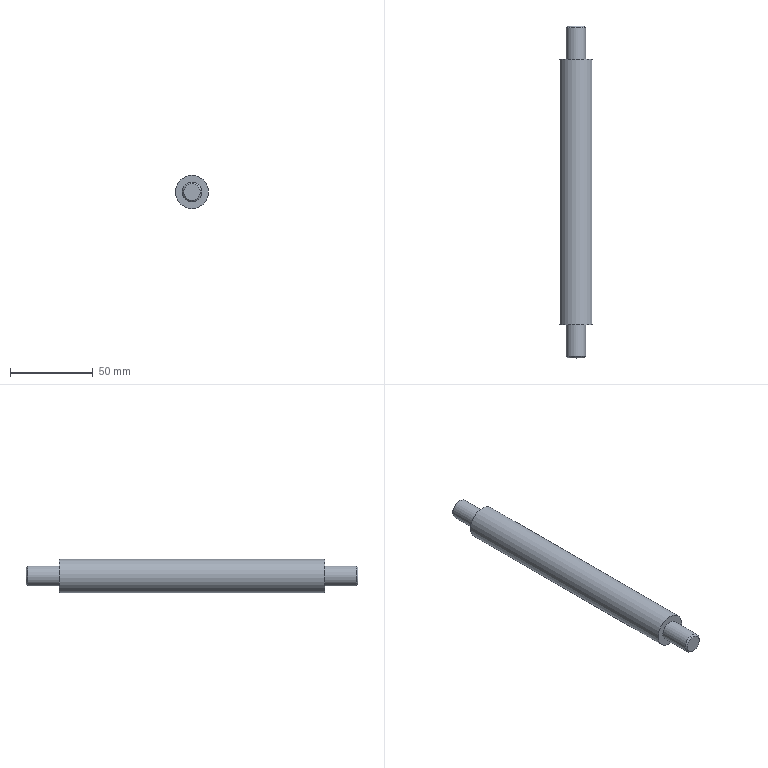Part | STEP file | 冲床-300配套压波_id754_x_t | 1 solid | 9 faces | box 20 x 200 x 20 mm | volume 54754 mm3 | plane 4 | cylinder 3 | cone 2 | commonest cylinder face diameters 12 x2 20 x1
STEP:
#1=CARTESIAN_POINT('',(1915.,80.,68.));
#2=VERTEX_POINT('',#1);
#3=CARTESIAN_POINT('',(1915.,80.,58.));
#4=DIRECTION('',(0.,1.,0.));
#5=DIRECTION('',(0.,0.,1.));
#6=AXIS2_PLACEMENT_3D('',#3,#4,#5);
#7=CIRCLE('',#6,10.);
#8=EDGE_CURVE('',#2,#2,#7,.T.);
#9=ORIENTED_EDGE('',*,*,#8,.F.);
#10=EDGE_LOOP('',(#9));
#11=FACE_BOUND('',#10,.T.);
#12=CARTESIAN_POINT('',(1915.,-80.,48.));
#13=VERTEX_POINT('',#12);
#14=CARTESIAN_POINT('',(1915.,-80.,58.));
#15=DIRECTION('',(0.,-1.,0.));
#16=DIRECTION('',(0.,0.,-1.));
#17=AXIS2_PLACEMENT_3D('',#14,#15,#16);
#18=CIRCLE('',#17,10.);
#19=EDGE_CURVE('',#13,#13,#18,.T.);
#20=ORIENTED_EDGE('',*,*,#19,.F.);
#21=EDGE_LOOP('',(#20));
#22=FACE_BOUND('',#21,.T.);
#23=CARTESIAN_POINT('',(1915.,-45.,58.));
#24=DIRECTION('',(0.,1.,0.));
#25=DIRECTION('',(0.,0.,-1.));
#26=AXIS2_PLACEMENT_3D('',#23,#24,#25);
#27=CYLINDRICAL_SURFACE('',#26,10.);
#28=ADVANCED_FACE('',(#11,#22),#27,.T.);
#29=CARTESIAN_POINT('',(1915.,80.,64.));
#30=VERTEX_POINT('',#29);
#31=CARTESIAN_POINT('',(1915.,80.,58.));
#32=DIRECTION('',(0.,-1.,0.));
#33=DIRECTION('',(0.,0.,1.));
#34=AXIS2_PLACEMENT_3D('',#31,#32,#33);
#35=CIRCLE('',#34,6.);
#36=EDGE_CURVE('',#30,#30,#35,.T.);
#37=ORIENTED_EDGE('',*,*,#36,.T.);
#38=EDGE_LOOP('',(#37));
#39=FACE_BOUND('',#38,.T.);
#40=ORIENTED_EDGE('',*,*,#8,.T.);
#41=EDGE_LOOP('',(#40));
#42=FACE_BOUND('',#41,.T.);
#43=CARTESIAN_POINT('',(1915.,80.,58.));
#44=DIRECTION('',(0.,1.,0.));
#45=DIRECTION('',(0.,0.,-1.));
#46=AXIS2_PLACEMENT_3D('',#43,#44,#45);
#47=PLANE('',#46);
#48=ADVANCED_FACE('',(#39,#42),#47,.T.);
#49=CARTESIAN_POINT('',(1915.,99.,52.));
#50=VERTEX_POINT('',#49);
#51=CARTESIAN_POINT('',(1915.,99.,58.));
#52=DIRECTION('',(0.,-1.,0.));
#53=DIRECTION('',(0.,0.,-1.));
#54=AXIS2_PLACEMENT_3D('',#51,#52,#53);
#55=CIRCLE('',#54,6.);
#56=EDGE_CURVE('',#50,#50,#55,.T.);
#57=ORIENTED_EDGE('',*,*,#56,.T.);
#58=EDGE_LOOP('',(#57));
#59=FACE_BOUND('',#58,.T.);
#60=ORIENTED_EDGE('',*,*,#36,.F.);
#61=EDGE_LOOP('',(#60));
#62=FACE_BOUND('',#61,.T.);
#63=CARTESIAN_POINT('',(1915.,105.,58.));
#64=DIRECTION('',(0.,-1.,0.));
#65=DIRECTION('',(0.,0.,1.));
#66=AXIS2_PLACEMENT_3D('',#63,#64,#65);
#67=CYLINDRICAL_SURFACE('',#66,6.);
#68=ADVANCED_FACE('',(#59,#62),#67,.T.);
#69=CARTESIAN_POINT('',(1920.,100.,58.));
#70=VERTEX_POINT('',#69);
#71=CARTESIAN_POINT('',(1915.,100.,58.));
#72=DIRECTION('',(0.,1.,0.));
#73=DIRECTION('',(1.,0.,0.));
#74=AXIS2_PLACEMENT_3D('',#71,#72,#73);
#75=CIRCLE('',#74,5.);
#76=EDGE_CURVE('',#70,#70,#75,.T.);
#77=ORIENTED_EDGE('',*,*,#76,.T.);
#78=EDGE_LOOP('',(#77));
#79=FACE_OUTER_BOUND('',#78,.T.);
#80=CARTESIAN_POINT('',(1940.,100.,-62.));
#81=DIRECTION('',(0.,-1.,0.));
#82=DIRECTION('',(0.,0.,1.));
#83=AXIS2_PLACEMENT_3D('',#80,#81,#82);
#84=PLANE('',#83);
#85=ADVANCED_FACE('',(#79),#84,.F.);
#86=CARTESIAN_POINT('',(1915.,-80.,52.));
#87=VERTEX_POINT('',#86);
#88=CARTESIAN_POINT('',(1915.,-80.,58.));
#89=DIRECTION('',(0.,1.,0.));
#90=DIRECTION('',(0.,0.,-1.));
#91=AXIS2_PLACEMENT_3D('',#88,#89,#90);
#92=CIRCLE('',#91,6.);
#93=EDGE_CURVE('',#87,#87,#92,.T.);
#94=ORIENTED_EDGE('',*,*,#93,.T.);
#95=EDGE_LOOP('',(#94));
#96=FACE_BOUND('',#95,.T.);
#97=ORIENTED_EDGE('',*,*,#19,.T.);
#98=EDGE_LOOP('',(#97));
#99=FACE_BOUND('',#98,.T.);
#100=CARTESIAN_POINT('',(1915.,-80.,58.));
#101=DIRECTION('',(0.,-1.,0.));
#102=DIRECTION('',(0.,0.,-1.));
#103=AXIS2_PLACEMENT_3D('',#100,#101,#102);
#104=PLANE('',#103);
#105=ADVANCED_FACE('',(#96,#99),#104,.T.);
#106=CARTESIAN_POINT('',(1915.,-99.,64.));
#107=VERTEX_POINT('',#106);
#108=CARTESIAN_POINT('',(1915.,-99.,58.));
#109=DIRECTION('',(0.,1.,0.));
#110=DIRECTION('',(0.,0.,1.));
#111=AXIS2_PLACEMENT_3D('',#108,#109,#110);
#112=CIRCLE('',#111,6.);
#113=EDGE_CURVE('',#107,#107,#112,.T.);
#114=ORIENTED_EDGE('',*,*,#113,.T.);
#115=EDGE_LOOP('',(#114));
#116=FACE_BOUND('',#115,.T.);
#117=ORIENTED_EDGE('',*,*,#93,.F.);
#118=EDGE_LOOP('',(#117));
#119=FACE_BOUND('',#118,.T.);
#120=CARTESIAN_POINT('',(1915.,-105.,58.));
#121=DIRECTION('',(0.,1.,0.));
#122=DIRECTION('',(0.,0.,1.));
#123=AXIS2_PLACEMENT_3D('',#120,#121,#122);
#124=CYLINDRICAL_SURFACE('',#123,6.);
#125=ADVANCED_FACE('',(#116,#119),#124,.T.);
#126=CARTESIAN_POINT('',(1915.,-100.,63.));
#127=VERTEX_POINT('',#126);
#128=CARTESIAN_POINT('',(1915.,-100.,58.));
#129=DIRECTION('',(0.,-1.,0.));
#130=DIRECTION('',(0.,0.,1.));
#131=AXIS2_PLACEMENT_3D('',#128,#129,#130);
#132=CIRCLE('',#131,5.);
#133=EDGE_CURVE('',#127,#127,#132,.T.);
#134=ORIENTED_EDGE('',*,*,#133,.T.);
#135=EDGE_LOOP('',(#134));
#136=FACE_OUTER_BOUND('',#135,.T.);
#137=CARTESIAN_POINT('',(1940.,-100.,-62.));
#138=DIRECTION('',(0.,1.,0.));
#139=DIRECTION('',(0.,0.,1.));
#140=AXIS2_PLACEMENT_3D('',#137,#138,#139);
#141=PLANE('',#140);
#142=ADVANCED_FACE('',(#136),#141,.F.);
#143=ORIENTED_EDGE('',*,*,#113,.F.);
#144=EDGE_LOOP('',(#143));
#145=FACE_BOUND('',#144,.T.);
#146=ORIENTED_EDGE('',*,*,#133,.F.);
#147=EDGE_LOOP('',(#146));
#148=FACE_BOUND('',#147,.T.);
#149=CARTESIAN_POINT('',(1915.,-100.,58.));
#150=DIRECTION('',(0.,1.,0.));
#151=DIRECTION('',(0.,0.,1.));
#152=AXIS2_PLACEMENT_3D('',#149,#150,#151);
#153=CONICAL_SURFACE('',#152,5.,45.);
#154=ADVANCED_FACE('',(#145,#148),#153,.T.);
#155=ORIENTED_EDGE('',*,*,#56,.F.);
#156=EDGE_LOOP('',(#155));
#157=FACE_BOUND('',#156,.T.);
#158=ORIENTED_EDGE('',*,*,#76,.F.);
#159=EDGE_LOOP('',(#158));
#160=FACE_BOUND('',#159,.T.);
#161=CARTESIAN_POINT('',(1915.,100.,58.));
#162=DIRECTION('',(0.,-1.,0.));
#163=DIRECTION('',(0.,0.,-1.));
#164=AXIS2_PLACEMENT_3D('',#161,#162,#163);
#165=CONICAL_SURFACE('',#164,5.,45.);
#166=ADVANCED_FACE('',(#157,#160),#165,.T.);
#167=CLOSED_SHELL('',(#28,#48,#68,#85,#105,#125,#142,#154,#166));
#168=MANIFOLD_SOLID_BREP('',#167);
#169=(LENGTH_UNIT()NAMED_UNIT(*)SI_UNIT(.MILLI.,.METRE.));
#170=UNCERTAINTY_MEASURE_WITH_UNIT(LENGTH_MEASURE(0.00002),#169,'','');
#171=(NAMED_UNIT(*)PLANE_ANGLE_UNIT()SI_UNIT($,.RADIAN.));
#172=PLANE_ANGLE_MEASURE_WITH_UNIT(PLANE_ANGLE_MEASURE(0.01745),#171);
#173=DIMENSIONAL_EXPONENTS(0.,0.,0.,0.,0.,0.,0.);
#174=(CONVERSION_BASED_UNIT('DEGREE',#172)NAMED_UNIT(#173)PLANE_ANGLE_UNIT());
#175=(NAMED_UNIT(*)SI_UNIT($,.STERADIAN.)SOLID_ANGLE_UNIT());
#176=(GEOMETRIC_REPRESENTATION_CONTEXT(3)GLOBAL_UNCERTAINTY_ASSIGNED_CONTEXT((#170))GLOBAL_UNIT_ASSIGNED_CONTEXT((#169,#174,#175))REPRESENTATION_CONTEXT('',''));
#177=ADVANCED_BREP_SHAPE_REPRESENTATION('',(#168),#176);